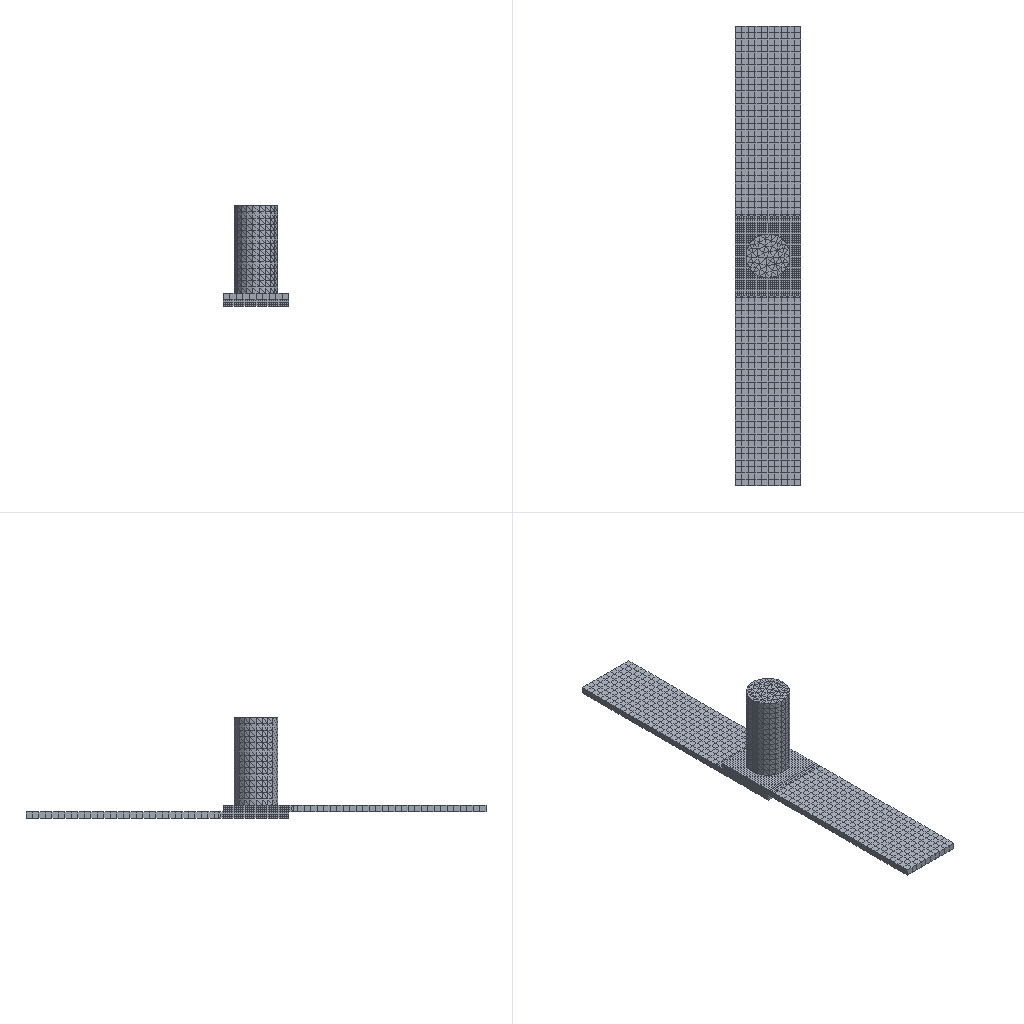Simulation study | abaqus
Set-up summary:
category,name,step,type,value,unit,region
solver,abaqus
solver,version,,,Abaqus/Explicit 2020
units,not stated in the deck,,not stated
analysis,deck,,dynamic temperature-displacement,dynamic temperature-displacement
load_step,Step-1,Step-1,dynamic temperature-displacement,nlgeom=True
contact,interactions,,,general=1 pairs=0 ties=0
load_step,requested,,,1
mesh,nodes,,,10125
mesh,elements,,,9730
element_type,C3D4T,,solid,3430
element_type,EC3D8RT,,solid,6300
load,load commands in deck,,count,3
bc,support commands in deck,,count,10
material,CFRTP,,in results
material,TOOL,,in results
check,setup vs results,,match,"per instance, exact: element labels, types and connectivity; labels of the nodes the elements use; coordinates of those nodes at SINGLE_PRECISION in 3 of 3 instance(s)"
Abaqus input file, long lists of numbers shortened:
*Heading
** Job name: Job-1 Model name: CFRTP1
** Generated by: Abaqus/CAE 2020
*Preprint, echo=NO, model=NO, history=NO, contact=NO
**
** PARTS
**
*Part, name=PLATE
*Node
      1, 0.03, 0.034, 0.003
      2, 0.03, 0.034,           0.
** (4666 more lines like these left out)
*Element, type=EC3D8RT
   1,    9,  213,  741,  489,    1,    2,   83,  138
   2,  489,  741,  742,  490,  138,   83,   84,  137
** (3148 more lines like these left out)
*Nset, nset=SET-1, generate
    1,  4668,     1
*Elset, elset=SET-1, generate
    1,  3150,     1
** Section: Section-1-SET-1
*Eulerian Section, elset=SET-1
CFRTP, CFRTP-2
*Surface, type=EULERIAN MATERIAL, name=CFRTP-2
CFRTP-2
*End Part
**
*Part, name=PLATE2
*Node
      1, 0.03, 0.034, 0.003
      2, 0.03, 0.034,           0.
** (4666 more lines like these left out)
*Element, type=EC3D8RT
   1,    9,  213,  741,  489,    1,    2,   83,  138
   2,  489,  741,  742,  490,  138,   83,   84,  137
** (3148 more lines like these left out)
*Nset, nset=SET-1, generate
    1,  4668,     1
*Elset, elset=SET-1, generate
    1,  3150,     1
** Section: Section-2-SET-1
*Eulerian Section, elset=SET-1
CFRTP, CFRTP-2
*Surface, type=EULERIAN MATERIAL, name=CFRTP-2
CFRTP-2
*End Part
**
*Part, name=TOOL
*Node
      1, 0.01,           0.,           0.
      2, 0.01,           0., 0.04
** (787 more lines like these left out)
*Element, type=C3D4T
   1, 399, 400, 401, 402
   2, 399, 403, 404, 405
** (3428 more lines like these left out)
*Nset, nset=SET-1, generate
   1,  789,    1
*Elset, elset=SET-1, generate
    1,  3430,     1
** Section: Section-3-SET-1
*Solid Section, elset=SET-1, material=TOOL
,
*End Part
**
**
** ASSEMBLY
**
*Assembly, name=Assembly
**
*Instance, name=PLATE-1, part=PLATE
*End Instance
**
*Instance, name=PLATE2-1, part=PLATE2
        0.03,         0.03,        0.003
        0.03,         0.03,        0.003,         0.03,         0.03,        1.003,         180.
*End Instance
**
*Instance, name=TOOL-1, part=TOOL
       0.015,        0.015,        0.006
*End Instance
**
*Node
      1, 0.025, 0.015, 0.046
*Nset, nset=B_SET-2, instance=TOOL-1, generate
   1,  789,    1
*Elset, elset=B_SET-2, instance=TOOL-1, generate
    1,  3430,     1
*Nset, nset=M_SET-1, instance=TOOL-1
 2,
*Nset, nset=SET-4, instance=PLATE-1
    3,    4,    6,    7,   20,   21,   25,   26,  195,  196,  197,  198,  199,  200,  201,  202
  203,  204,  205,  206,  207,  208,  209,  210,  211,  212,  253,  254,  313,  314,  344,  345
** (8 more lines like these left out)
*Nset, nset=SET-4, instance=PLATE2-1
    3,    4,    6,    7,   20,   21,   25,   26,  195,  196,  197,  198,  199,  200,  201,  202
  203,  204,  205,  206,  207,  208,  209,  210,  211,  212,  253,  254,  313,  314,  344,  345
** (8 more lines like these left out)
*Elset, elset=SET-4, instance=PLATE-1
   29,   58,   87,  116,  145,  174,  203,  232,  261,  290,  378,  379,  380,  468,  469,  470
  558,  559,  560,  648,  649,  650,  738,  739,  740,  828,  829,  830,  918,  919,  920, 1008
** (5 more lines like these left out)
*Elset, elset=SET-4, instance=PLATE2-1
   29,   58,   87,  116,  145,  174,  203,  232,  261,  290,  378,  379,  380,  468,  469,  470
  558,  559,  560,  648,  649,  650,  738,  739,  740,  828,  829,  830,  918,  919,  920, 1008
** (5 more lines like these left out)
*Nset, nset=SET-5, instance=PLATE-1
    1,    2,    3,    4,    5,    6,    7,    8,   18,   19,   20,   21,   22,   23,   24,   25
   26,   27,   28,   29,   30,   31,   32,   33,   83,   84,   85,   86,   87,   88,   89,   90
** (22 more lines like these left out)
*Nset, nset=SET-5, instance=PLATE2-1
    1,    2,    3,    4,    5,    6,    7,    8,   18,   19,   20,   21,   22,   23,   24,   25
   26,   27,   28,   29,   30,   31,   32,   33,   83,   84,   85,   86,   87,   88,   89,   90
** (22 more lines like these left out)
*Elset, elset=SET-5, instance=PLATE-1
    1,    2,    3,    4,    5,    6,    7,    8,    9,   10,   11,   12,   13,   14,   15,   16
   17,   18,   19,   20,   21,   22,   23,   24,   25,   26,   27,   28,   29,  262,  263,  264
** (14 more lines like these left out)
*Elset, elset=SET-5, instance=PLATE2-1
    1,    2,    3,    4,    5,    6,    7,    8,    9,   10,   11,   12,   13,   14,   15,   16
   17,   18,   19,   20,   21,   22,   23,   24,   25,   26,   27,   28,   29,  262,  263,  264
** (14 more lines like these left out)
*Nset, nset=SET-6, instance=PLATE-1
    1,    2,    3,    4,    5,    6,    7,    8,    9,   10,   11,   12,   13,   14,   15,   16
   17,   18,   19,   20,   24,   25,   27,   28,   31,   32,   33,   34,   35,   36,   37,   38
** (107 more lines like these left out)
*Nset, nset=SET-6, instance=PLATE2-1
    1,    2,    3,    4,    5,    6,    7,    8,    9,   10,   11,   12,   13,   14,   15,   16
   17,   18,   21,   26,   27,   28,   31,   32,   33,   34,   35,   36,   37,   38,   39,   40
** (105 more lines like these left out)
*Elset, elset=SET-6, instance=PLATE-1
    1,    2,    3,    4,    5,    6,    7,    8,    9,   10,   11,   12,   13,   14,   15,   16
   17,   18,   19,   20,   21,   22,   23,   24,   25,   26,   27,   28,   29,   30,   31,   32
** (79 more lines like these left out)
*Elset, elset=SET-6, instance=PLATE2-1
    1,    2,    3,    4,    5,    6,    7,    8,    9,   10,   11,   12,   13,   14,   15,   16
   17,   18,   19,   20,   21,   22,   23,   24,   25,   26,   27,   28,   29,   30,   31,   32
** (77 more lines like these left out)
*Nset, nset=SET-7, instance=PLATE-1, generate
    1,  4668,     1
*Nset, nset=SET-7, instance=PLATE2-1, generate
    1,  4668,     1
*Elset, elset=SET-7, instance=PLATE-1, generate
    1,  3150,     1
*Elset, elset=SET-7, instance=PLATE2-1, generate
    1,  3150,     1
*Nset, nset=SET-8, instance=TOOL-1
   1,   2,   3,   4,   5,   6,   7,   8,   9,  10,  11,  12,  13,  14,  15,  16
  17,  18,  19,  20,  21,  22,  23,  24,  25,  26,  27,  28,  29,  30,  31,  32
** (19 more lines like these left out)
*Elset, elset=SET-8, instance=TOOL-1
   50,   81,   86,   87,  104,  113,  132,  137,  175,  195,  202,  226,  258,  259,  336,  341
  373,  384,  404,  429,  435,  469,  531,  558,  585,  598,  600,  636,  642,  708,  709,  714
** (37 more lines like these left out)
*Nset, nset=SET-9, instance=PLATE2-1
   18,   19,   20,   21,   22,   23,   24,   25,   26,   27,  222,  223,  224,  225,  226,  227
  228,  229,  230,  231,  232,  233,  234,  235,  236,  237,  238,  239,  240,  241,  242,  243
** (239 more lines like these left out)
*Elset, elset=SET-9, instance=PLATE2-1, generate
  291,  2990,     1
*Nset, nset=SET-10, instance=PLATE-1
   18,   19,   20,   21,   22,   23,   24,   25,   26,   27,  222,  223,  224,  225,  226,  227
  228,  229,  230,  231,  232,  233,  234,  235,  236,  237,  238,  239,  240,  241,  242,  243
** (239 more lines like these left out)
*Elset, elset=SET-10, instance=PLATE-1, generate
  291,  2990,     1
*Nset, nset=SET-11, instance=PLATE2-1, generate
    1,  4668,     1
*Elset, elset=SET-11, instance=PLATE2-1, generate
    1,  3150,     1
*Nset, nset=SET-12, instance=PLATE-1, generate
    1,  4668,     1
*Elset, elset=SET-12, instance=PLATE-1, generate
    1,  3150,     1
*Nset, nset=SET-13, instance=TOOL-1, generate
   1,  789,    1
*Elset, elset=SET-13, instance=TOOL-1, generate
    1,  3430,     1
*Nset, nset=SURFACE1, instance=PLATE-1
   18,   21,   26,   27,  255,  256,  257,  258,  259,  260,  261,  262,  263,  264,  265,  266
  267,  268,  269,  270,  271,  272,  273,  274,  275,  276,  277,  278,  279,  280,  281,  282
** (59 more lines like these left out)
*Elset, elset=SURFACE1, instance=PLATE-1, generate
  291,  2988,     3
*Nset, nset=SURFACE2, instance=PLATE2-1
   19,   20,   24,   25,  224,  225,  226,  227,  228,  229,  230,  231,  232,  233,  234,  235
  236,  237,  238,  239,  240,  241,  242,  243,  244,  245,  246,  247,  248,  249,  250,  251
** (59 more lines like these left out)
*Elset, elset=SURFACE2, instance=PLATE2-1, generate
  293,  2990,     3
*Nset, nset=SURFACE3, instance=TOOL-1
  1,  3,  4,  5,  6,  7,  8,  9, 10, 11, 12, 13, 14, 15, 16, 17
 18, 19, 20, 21, 22, 23, 45, 46, 47, 48, 49, 50, 51, 52, 53, 54
** (2 more lines like these left out)
*Elset, elset=SURFACE3, instance=TOOL-1
  320,  761, 1058, 1084, 1109, 1336, 1579, 1618, 1650, 1652, 1663, 1664, 1674, 1680, 1697, 1709
 1717, 1736, 1742, 1743, 1752, 1758, 1770, 1777, 1792, 1795, 1804, 1809, 1826, 1840, 1843, 1844
** (4 more lines like these left out)
*Nset, nset=Set-37, instance=PLATE-1
    2,    3,    5,    6,   19,   20,   24,   25,   28,   33,   83,   84,   85,   86,   87,   88
   89,   90,   91,   92,   93,   94,   95,   96,   97,   98,   99,  100,  101,  102,  103,  104
** (82 more lines like these left out)
*Nset, nset=Set-38, instance=PLATE2-1
   3,   4,   6,   7, 195, 196, 197, 198, 199, 200, 201, 202, 203, 204, 205, 206
 207, 208, 209, 210, 211, 212
*Nset, nset=Set-38, instance=PLATE-1
   3,   4,   6,   7, 195, 196, 197, 198, 199, 200, 201, 202, 203, 204, 205, 206
 207, 208, 209, 210, 211, 212
*Nset, nset=Set-39
 1,
*Nset, nset=_PICKEDSET19, internal
 1,
*Nset, nset=_PickedSet78, internal
 1,
*Elset, elset=_SURF-1_S2, internal, instance=PLATE-1, generate
 3111,  3150,     1
*Elset, elset=_SURF-1_S2, internal, instance=PLATE2-1, generate
 3111,  3150,     1
*Elset, elset=_SURF-1_S4, internal, instance=PLATE-1
    1,    2,    3,    4,    5,    6,    7,    8,    9,   10,   11,   12,   13,   14,   15,   16
   17,   18,   19,   20,   21,   22,   23,   24,   25,   26,   27,   28,   29,   30,   31,   32
** (75 more lines like these left out)
*Elset, elset=_SURF-1_S4, internal, instance=PLATE2-1
    1,    2,    3,    4,    5,    6,    7,    8,    9,   10,   11,   12,   13,   14,   15,   16
   17,   18,   19,   20,   21,   22,   23,   24,   25,   26,   27,   28,   29,   30,   31,   32
** (18 more lines like these left out)
*Elset, elset=_SURF-1_S5, internal, instance=PLATE-1
  378,  379,  380,  468,  469,  470,  558,  559,  560,  648,  649,  650,  738,  739,  740,  828
  829,  830,  918,  919,  920, 1008, 1009, 1010, 1098, 1099, 1100, 1188, 1189, 1190, 1278, 1279
** (4 more lines like these left out)
*Elset, elset=_SURF-2_S1, internal, instance=PLATE-1
  262,  263,  264,  265,  266,  267,  268,  269,  270,  271,  272,  273,  274,  275,  276,  277
  278,  279,  280,  281,  282,  283,  284,  285,  286,  287,  288,  289,  290, 2901, 2902, 2903
** (9 more lines like these left out)
*Elset, elset=_SURF-2_S1, internal, instance=PLATE2-1
  262,  263,  264,  265,  266,  267,  268,  269,  270,  271,  272,  273,  274,  275,  276,  277
  278,  279,  280,  281,  282,  283,  284,  285,  286,  287,  288,  289,  290, 2901, 2902, 2903
** (9 more lines like these left out)
*Elset, elset=_SURF-2_S2, internal, instance=PLATE-1
    1,    2,    3,    4,    5,    6,    7,    8,    9,   10,   11,   12,   13,   14,   15,   16
   17,   18,   19,   20,   21,   22,   23,   24,   25,   26,   27,   28,   29,  291,  292,  293
** (6 more lines like these left out)
*Elset, elset=_SURF-2_S2, internal, instance=PLATE2-1
    1,    2,    3,    4,    5,    6,    7,    8,    9,   10,   11,   12,   13,   14,   15,   16
   17,   18,   19,   20,   21,   22,   23,   24,   25,   26,   27,   28,   29,  291,  292,  293
** (6 more lines like these left out)
*Elset, elset=_SURF-2_S3, internal, instance=PLATE-1
 3120, 3145
*Elset, elset=_SURF-2_S3, internal, instance=PLATE2-1
 3120, 3145
*Elset, elset=_SURF-2_S5, internal, instance=PLATE2-1
  378,  379,  380,  468,  469,  470,  558,  559,  560,  648,  649,  650,  738,  739,  740,  828
  829,  830,  918,  919,  920, 1008, 1009, 1010, 1098, 1099, 1100, 1188, 1189, 1190, 1278, 1279
** (4 more lines like these left out)
*Elset, elset=_SURF-2_S6, internal, instance=PLATE-1
    1,    2,    3,    4,    5,    6,    7,    8,    9,   10,   11,   12,   13,   14,   15,   16
   17,   18,   19,   20,   21,   22,   23,   24,   25,   26,   27,   28,   29,   30,   31,   32
** (18 more lines like these left out)
*Elset, elset=_SURF-2_S6, internal, instance=PLATE2-1
    1,    2,    3,    4,    5,    6,    7,    8,    9,   10,   11,   12,   13,   14,   15,   16
   17,   18,   19,   20,   21,   22,   23,   24,   25,   26,   27,   28,   29,   30,   31,   32
** (75 more lines like these left out)
*Elset, elset=_SURF-4_S1, internal, instance=TOOL-1
 1650, 1843, 3382
*Elset, elset=_SURF-4_S2, internal, instance=TOOL-1
 1858, 1865, 1940, 3047, 3104, 3330
*Elset, elset=_SURF-4_S3, internal, instance=TOOL-1
  320,  761, 1084, 1109, 1579, 1618, 1652, 1663, 1664, 1674, 1680, 1697, 1709, 1717, 1736, 1743
 1752, 1758, 1770, 1777, 1792, 1795, 1804, 1809, 1826, 1840, 1844, 1850, 1856, 1867, 1884, 1908
** (3 more lines like these left out)
*Elset, elset=_SURF-4_S4, internal, instance=TOOL-1
 1058, 1336, 1742, 1862, 1950, 2431, 3075, 3099, 3136, 3414
*Elset, elset=_SURF-5_S6, internal, instance=PLATE2-1, generate
  291,  2988,     3
*Elset, elset=_SURF-6_S6, internal, instance=PLATE-1, generate
  291,  2988,     3
*Elset, elset=_SURF-7_S4, internal, instance=PLATE2-1, generate
  293,  2990,     3
*Elset, elset=_S_SURF-3_S1, internal, instance=TOOL-1
   50,   87,  104,  558,  709,  731, 1316, 1524, 1587, 1596, 1650, 1843, 1898, 1922, 1940, 2029
 2107, 2160, 2277, 2335, 2406, 2558, 2703, 2737, 2816, 2923, 2979, 3045, 3047, 3064, 3079, 3094
** (1 more lines like these left out)
*Elset, elset=_S_SURF-3_S2, internal, instance=TOOL-1
 1196, 1582, 1605, 1668, 1858, 1865, 1925, 1940, 1990, 1993, 2010, 2042, 2106, 2116, 2130, 2146
 2157, 2169, 2740, 2742, 2752, 2759, 2780, 2787, 2864, 2882, 2899, 2920, 3035, 3047, 3104, 3116
** (1 more lines like these left out)
*Elset, elset=_S_SURF-3_S3, internal, instance=TOOL-1
   72,   81,   86,  113,  132,  137,  175,  195,  202,  226,  258,  259,  320,  336,  341,  373
  384,  404,  417,  418,  429,  435,  469,  500,  519,  531,  558,  585,  598,  600,  616,  625
** (39 more lines like these left out)
*Elset, elset=_S_SURF-3_S4, internal, instance=TOOL-1
  104,  733,  968, 1058, 1126, 1184, 1245, 1336, 1549, 1585, 1591, 1659, 1709, 1739, 1742, 1785
 1786, 1840, 1841, 1862, 1867, 1906, 1923, 1950, 2037, 2072, 2093, 2169, 2236, 2241, 2245, 2415
** (1 more lines like these left out)
*Elset, elset=_SURF-1_S2_1, internal, instance=PLATE-1, generate
 3111,  3150,     1
*Elset, elset=_SURF-1_S2_1, internal, instance=PLATE2-1, generate
 3111,  3150,     1
*Elset, elset=_SURF-1_S4_1, internal, instance=PLATE-1
    1,    2,    3,    4,    5,    6,    7,    8,    9,   10,   11,   12,   13,   14,   15,   16
   17,   18,   19,   20,   21,   22,   23,   24,   25,   26,   27,   28,   29,   30,   31,   32
** (75 more lines like these left out)
*Elset, elset=_SURF-1_S4_1, internal, instance=PLATE2-1
    1,    2,    3,    4,    5,    6,    7,    8,    9,   10,   11,   12,   13,   14,   15,   16
   17,   18,   19,   20,   21,   22,   23,   24,   25,   26,   27,   28,   29,   30,   31,   32
** (18 more lines like these left out)
*Elset, elset=_SURF-1_S5_1, internal, instance=PLATE-1
  378,  379,  380,  468,  469,  470,  558,  559,  560,  648,  649,  650,  738,  739,  740,  828
  829,  830,  918,  919,  920, 1008, 1009, 1010, 1098, 1099, 1100, 1188, 1189, 1190, 1278, 1279
** (4 more lines like these left out)
*Surface, type=ELEMENT, name=SURF-1
_SURF-1_S2_1, S2
_SURF-1_S4_1, S4
_SURF-1_S5_1, S5
*Elset, elset=_SURF-2_S3_1, internal, instance=PLATE-1
 3120, 3145
*Elset, elset=_SURF-2_S3_1, internal, instance=PLATE2-1
 3120, 3145
*Elset, elset=_SURF-2_S2_1, internal, instance=PLATE-1
    1,    2,    3,    4,    5,    6,    7,    8,    9,   10,   11,   12,   13,   14,   15,   16
   17,   18,   19,   20,   21,   22,   23,   24,   25,   26,   27,   28,   29,  291,  292,  293
** (6 more lines like these left out)
*Elset, elset=_SURF-2_S2_1, internal, instance=PLATE2-1
    1,    2,    3,    4,    5,    6,    7,    8,    9,   10,   11,   12,   13,   14,   15,   16
   17,   18,   19,   20,   21,   22,   23,   24,   25,   26,   27,   28,   29,  291,  292,  293
** (6 more lines like these left out)
*Elset, elset=_SURF-2_S6_1, internal, instance=PLATE-1
    1,    2,    3,    4,    5,    6,    7,    8,    9,   10,   11,   12,   13,   14,   15,   16
   17,   18,   19,   20,   21,   22,   23,   24,   25,   26,   27,   28,   29,   30,   31,   32
** (18 more lines like these left out)
*Elset, elset=_SURF-2_S6_1, internal, instance=PLATE2-1
    1,    2,    3,    4,    5,    6,    7,    8,    9,   10,   11,   12,   13,   14,   15,   16
   17,   18,   19,   20,   21,   22,   23,   24,   25,   26,   27,   28,   29,   30,   31,   32
** (75 more lines like these left out)
*Elset, elset=_SURF-2_S1_1, internal, instance=PLATE-1
  262,  263,  264,  265,  266,  267,  268,  269,  270,  271,  272,  273,  274,  275,  276,  277
  278,  279,  280,  281,  282,  283,  284,  285,  286,  287,  288,  289,  290, 2901, 2902, 2903
** (9 more lines like these left out)
*Elset, elset=_SURF-2_S1_1, internal, instance=PLATE2-1
  262,  263,  264,  265,  266,  267,  268,  269,  270,  271,  272,  273,  274,  275,  276,  277
  278,  279,  280,  281,  282,  283,  284,  285,  286,  287,  288,  289,  290, 2901, 2902, 2903
** (9 more lines like these left out)
*Elset, elset=_SURF-2_S5_1, internal, instance=PLATE2-1
  378,  379,  380,  468,  469,  470,  558,  559,  560,  648,  649,  650,  738,  739,  740,  828
  829,  830,  918,  919,  920, 1008, 1009, 1010, 1098, 1099, 1100, 1188, 1189, 1190, 1278, 1279
** (4 more lines like these left out)
*Surface, type=ELEMENT, name=SURF-2
_SURF-2_S3_1, S3
_SURF-2_S2_1, S2
_SURF-2_S6_1, S6
_SURF-2_S1_1, S1
_SURF-2_S5_1, S5
*Elset, elset=_SURF-4_S3_1, internal, instance=TOOL-1
  320,  761, 1084, 1109, 1579, 1618, 1652, 1663, 1664, 1674, 1680, 1697, 1709, 1717, 1736, 1743
 1752, 1758, 1770, 1777, 1792, 1795, 1804, 1809, 1826, 1840, 1844, 1850, 1856, 1867, 1884, 1908
** (3 more lines like these left out)
*Elset, elset=_SURF-4_S4_1, internal, instance=TOOL-1
 1058, 1336, 1742, 1862, 1950, 2431, 3075, 3099, 3136, 3414
*Elset, elset=_SURF-4_S2_1, internal, instance=TOOL-1
 1858, 1865, 1940, 3047, 3104, 3330
*Elset, elset=_SURF-4_S1_1, internal, instance=TOOL-1
 1650, 1843, 3382
*Surface, type=ELEMENT, name=SURF-4
_SURF-4_S3_1, S3
_SURF-4_S4_1, S4
_SURF-4_S2_1, S2
_SURF-4_S1_1, S1
*Surface, type=ELEMENT, name=SURF-5
_SURF-5_S6, S6
*Surface, type=ELEMENT, name=SURF-6
_SURF-6_S6, S6
*Surface, type=ELEMENT, name=SURF-7
_SURF-7_S4, S4
*Elset, elset=_S_SURF-3_S1_1, internal, instance=TOOL-1
   50,   87,  104,  558,  709,  731, 1316, 1524, 1587, 1596, 1650, 1843, 1898, 1922, 1940, 2029
 2107, 2160, 2277, 2335, 2406, 2558, 2703, 2737, 2816, 2923, 2979, 3045, 3047, 3064, 3079, 3094
** (1 more lines like these left out)
*Elset, elset=_S_SURF-3_S3_1, internal, instance=TOOL-1
   72,   81,   86,  113,  132,  137,  175,  195,  202,  226,  258,  259,  320,  336,  341,  373
  384,  404,  417,  418,  429,  435,  469,  500,  519,  531,  558,  585,  598,  600,  616,  625
** (39 more lines like these left out)
*Elset, elset=_S_SURF-3_S4_1, internal, instance=TOOL-1
  104,  733,  968, 1058, 1126, 1184, 1245, 1336, 1549, 1585, 1591, 1659, 1709, 1739, 1742, 1785
 1786, 1840, 1841, 1862, 1867, 1906, 1923, 1950, 2037, 2072, 2093, 2169, 2236, 2241, 2245, 2415
** (1 more lines like these left out)
*Elset, elset=_S_SURF-3_S2_1, internal, instance=TOOL-1
 1196, 1582, 1605, 1668, 1858, 1865, 1925, 1940, 1990, 1993, 2010, 2042, 2106, 2116, 2130, 2146
 2157, 2169, 2740, 2742, 2752, 2759, 2780, 2787, 2864, 2882, 2899, 2920, 3035, 3047, 3104, 3116
** (1 more lines like these left out)
*Surface, type=ELEMENT, name=S_SURF-3
_S_SURF-3_S1_1, S1
_S_SURF-3_S3_1, S3
_S_SURF-3_S4_1, S4
_S_SURF-3_S2_1, S2
** Constraint: RigidBody-1
*Rigid Body, ref node=_PickedSet78, elset=B_SET-2
*End Assembly
*Amplitude, name=AMP-1, definition=PERIODIC
1,         125600.,              0.,             0.5
             4.,              0.
**
** MATERIALS
**
*Material, name=CFRTP
*Conductivity
 0.427, 20.
 0.435,100.
 0.512,200.
*Density
1150.,
*Elastic, moduli=LONG TERM
 1.13e+10,  0.28,   20.
 5.35e+08,  0.28,  100.
  4.2e+09,  0.28,  200.
   20000.,   0.2,  300.
     100., 0.001,  400.
*Expansion
 3.5e-05,
*Specific Heat
1310., 20.
1950.,100.
2860.,200.
*Viscoelastic, frequency=PRONY
 0.999, 0.999, 0.001
*Material, name=TOOL
*Conductivity
 24.3,
*Density
7800.,
*Elastic
 2.1e+11, 0.3
*Specific Heat
460.,
**
** INTERACTION PROPERTIES
**
*Surface Interaction, name=FRICTION
*Friction
  0.3,  0., 0.1
 0.35,  0., 0.2
  0.4,  0., 0.3
 0.45,  0., 0.4
  0.5,  0., 0.5
*Surface Behavior, pressure-overclosure=HARD
*Contact Damping, definition=DAMPING COEFFICIENT
1.,
*Gap Conductance, pressure
 0.1,0.
 0.3,1.
*Gap Heat Generation
0.2, 0.1
*Surface Interaction, name="TOOL and plate"
*Friction
 0.2,
*Surface Behavior, pressure-overclosure=HARD
*Gap Conductance
 0.5,   0.
  0., 0.01
*Gap Heat Generation
0.1, 0.1
**
** PHYSICAL CONSTANTS
**
*Physical Constants, absolute zero=-273.15, stefan boltzmann=5.67e-08
**
** PREDEFINED FIELDS
**
** Name: Field-1   Type: Temperature
*Initial Conditions, type=TEMPERATURE
SET-7, 20.
** Name: Field-2   Type: Temperature
*Initial Conditions, type=TEMPERATURE
SET-13, 20.
** Name: VolumeFraction-1   Type: Material assignment
*Initial Conditions, type=VOLUME FRACTION
SET-11, PLATE2-1.CFRTP-2, 1.
** Name: VolumeFraction-2   Type: Material assignment
*Initial Conditions, type=VOLUME FRACTION
SET-12, PLATE-1.CFRTP-2, 1.
**
** INTERACTIONS
**
** Interaction: general_contact
*Contact, op=NEW
*Contact Inclusions, ALL EXTERIOR
*Contact Property Assignment
 ,  , FRICTION
*Contact Formulation, type=PURE MASTER-SLAVE
SURF-4 , SURF-5 , SLAVE
SURF-7 , SURF-6 , SLAVE
** ----------------------------------------------------------------
**
** STEP: Step-1
**
*Step, name=Step-1, nlgeom=YES
*Dynamic Temperature-displacement, Explicit
, 0.01
*Bulk Viscosity
0.06, 1.2
** Mass Scaling: Semi-Automatic
**               Whole Model
*Fixed Mass Scaling, factor=5000.
**
** BOUNDARY CONDITIONS
**
** Name: BC-1 Type: 对称/反对称/完全固定
*Boundary
Set-37, ENCASTRE
** Name: BC-2 Type: 对称/反对称/完全固定
*Boundary
Set-38, ENCASTRE
** Name: [REDACTED] : Velocity/Angular velocity
*Boundary, amplitude=AMP-1, type=VELOCITY
Set-39, 1, 1
Set-39, 2, 2
Set-39, 3, 3, -1.
Set-39, 4, 4
Set-39, 5, 5
Set-39, 6, 6
**
** INTERACTIONS
**
** Interaction: SURFFILM-1
*Sfilm
SURF-2, F, 20., 400.
** Interaction: SURFFILM-2
*Sfilm
SURF-1, F, 20., 100000.
**
** OUTPUT REQUESTS
**
*Restart, write, number interval=1, time marks=NO
**
** FIELD OUTPUT: F-Output-1
**
*Output, field, number interval=100
*Node Output
A, CF, COORD, NT, RF, RFL, RM, RT
U, V
*Element Output, directions=YES
E, EVF, EVOL, HFL, IVOL, LE, MISES, MISESMAX, MISESONLY, PE, PEEQ, PEEQMAX, PEEQT, PEEQVAVG, PEMAG, PEVAVG
S, SF, SSAVG, STATUS, STH, SVAVG, SVOL, TEMP
*Contact Output
CDISP, CSTRESS
*Output, history, frequency=0
*End Step
Results summary:
result,step,Step-1,completed,increments=68640 time=0.01/0.01
result,analysis,,,"dynamic temperature-displacement, explict"
result,last_loadstep,,,1
result,analysis steps,,count,1
result,primary field,,,"U, NT11"
result,reaction total,,FX,45.262,model units
result,reaction total,,FY,-47.143,model units
result,reaction total,,FZ,-144478924.742,model units